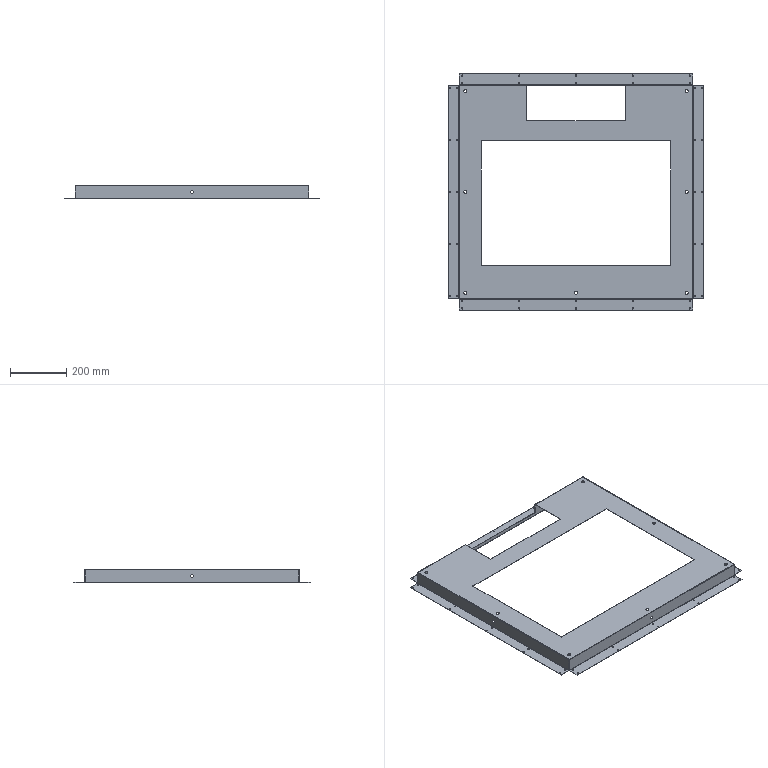Part | 1 solid | 184 faces | box 913 x 843 x 48 mm | volume 553017 mm3 | cylinder 118 | plane 58 | spline 8 | commonest cylinder face diameters 4.2 x80 11 x14 0.4 x9 2.4 x9 10 x6